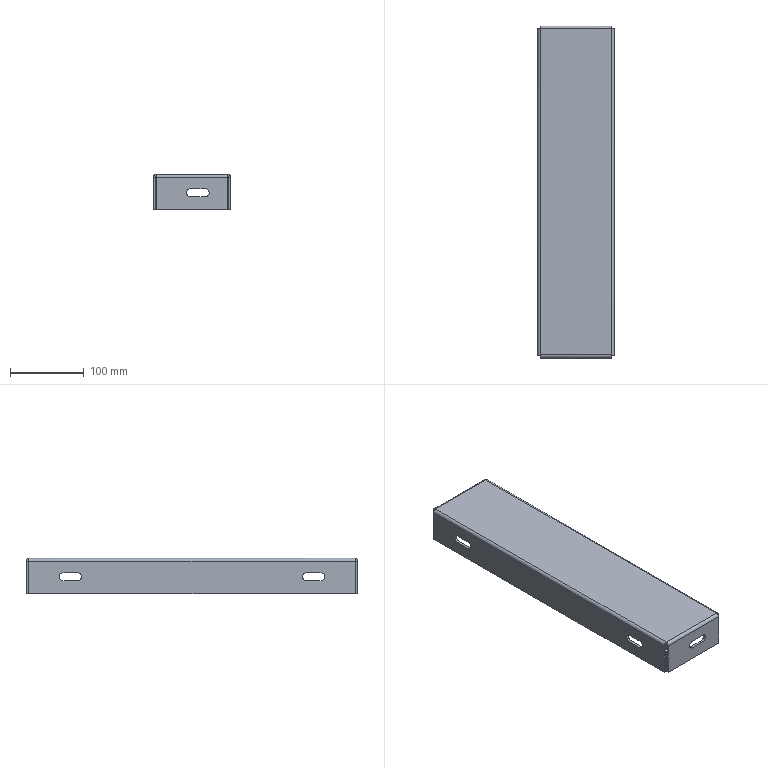Part | NX | features BREP 1 | 1 solid | 62 faces | box 104.1 x 449 x 48 mm | volume 276574 mm3 | plane 34 | cylinder 20 | spline 8 | commonest cylinder face diameters 10.5 x12 2 x4 8 x4